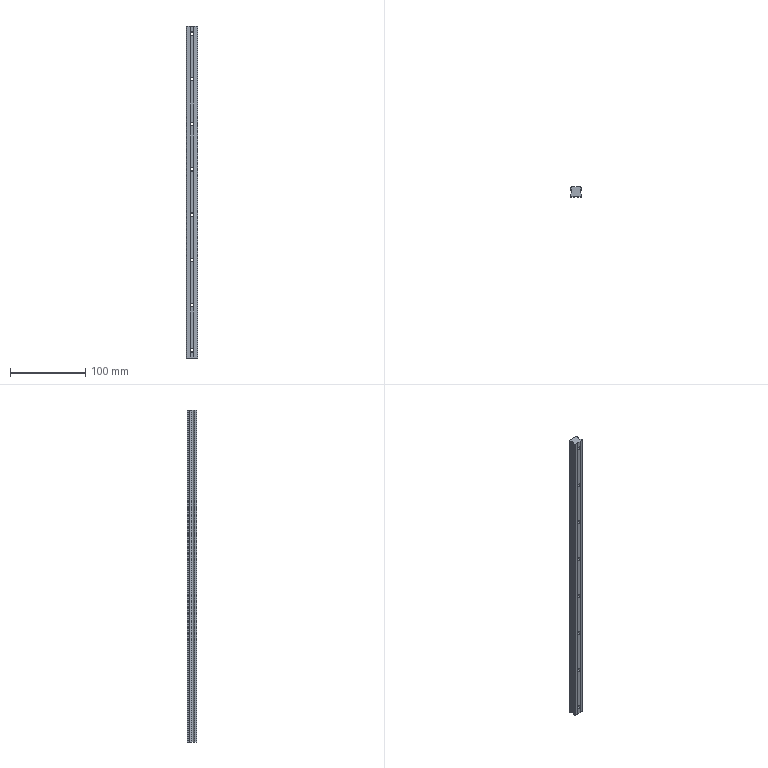Part | SolidWorks | features ICE 2, BaseBody 1, HoleWzd 1 | 1 solid | 86 faces | box 15 x 12.5 x 440 mm | volume 69027 mm3 | cylinder 50 | plane 36 | commonest cylinder face diameters 4.5 x16 8 x16 0.6 x11 3 x5 1 x2